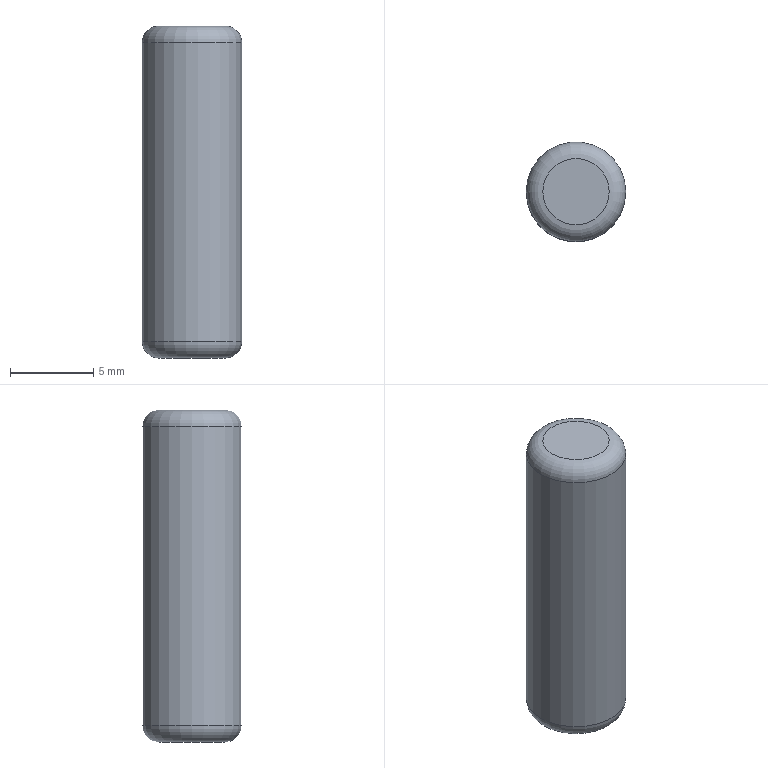Part | STEP file | 200 mesh_id710_x | 1 solid | 5 faces | box 6 x 6 x 20 mm | volume 557.999 mm3 | plane 2 | torus 2 | cylinder 1 | commonest cylinder face diameters 6 x1
STEP:
#1=CARTESIAN_POINT('',(-16807.686,-4170.269,20.));
#2=VERTEX_POINT('',#1);
#3=CARTESIAN_POINT('',(-16809.686,-4170.269,20.));
#4=DIRECTION('',(0.,0.,1.));
#5=DIRECTION('',(1.,0.,0.));
#6=AXIS2_PLACEMENT_3D('',#3,#4,#5);
#7=CIRCLE('',#6,2.);
#8=EDGE_CURVE('',#2,#2,#7,.T.);
#9=ORIENTED_EDGE('',*,*,#8,.T.);
#10=EDGE_LOOP('',(#9));
#11=FACE_OUTER_BOUND('',#10,.T.);
#12=CARTESIAN_POINT('',(-16809.686,-4170.269,20.));
#13=DIRECTION('',(0.,0.,1.));
#14=DIRECTION('',(1.,0.,0.));
#15=AXIS2_PLACEMENT_3D('',#12,#13,#14);
#16=PLANE('',#15);
#17=ADVANCED_FACE('',(#11),#16,.T.);
#18=CARTESIAN_POINT('',(-16811.686,-4170.269,0.));
#19=VERTEX_POINT('',#18);
#20=CARTESIAN_POINT('',(-16809.686,-4170.269,0.));
#21=DIRECTION('',(0.,0.,-1.));
#22=DIRECTION('',(-1.,0.,0.));
#23=AXIS2_PLACEMENT_3D('',#20,#21,#22);
#24=CIRCLE('',#23,2.);
#25=EDGE_CURVE('',#19,#19,#24,.T.);
#26=ORIENTED_EDGE('',*,*,#25,.T.);
#27=EDGE_LOOP('',(#26));
#28=FACE_OUTER_BOUND('',#27,.T.);
#29=CARTESIAN_POINT('',(-16809.686,-4170.269,0.));
#30=DIRECTION('',(0.,0.,-1.));
#31=DIRECTION('',(-1.,0.,0.));
#32=AXIS2_PLACEMENT_3D('',#29,#30,#31);
#33=PLANE('',#32);
#34=ADVANCED_FACE('',(#28),#33,.T.);
#35=CARTESIAN_POINT('',(-16812.686,-4170.269,1.));
#36=VERTEX_POINT('',#35);
#37=CARTESIAN_POINT('',(-16809.686,-4170.269,1.));
#38=DIRECTION('',(0.,0.,1.));
#39=DIRECTION('',(-1.,0.,0.));
#40=AXIS2_PLACEMENT_3D('',#37,#38,#39);
#41=CIRCLE('',#40,3.);
#42=EDGE_CURVE('',#36,#36,#41,.T.);
#43=ORIENTED_EDGE('',*,*,#42,.T.);
#44=EDGE_LOOP('',(#43));
#45=FACE_BOUND('',#44,.T.);
#46=CARTESIAN_POINT('',(-16806.686,-4170.269,19.));
#47=VERTEX_POINT('',#46);
#48=CARTESIAN_POINT('',(-16809.686,-4170.269,19.));
#49=DIRECTION('',(0.,0.,-1.));
#50=DIRECTION('',(1.,0.,0.));
#51=AXIS2_PLACEMENT_3D('',#48,#49,#50);
#52=CIRCLE('',#51,3.);
#53=EDGE_CURVE('',#47,#47,#52,.T.);
#54=ORIENTED_EDGE('',*,*,#53,.T.);
#55=EDGE_LOOP('',(#54));
#56=FACE_BOUND('',#55,.T.);
#57=CARTESIAN_POINT('',(-16809.686,-4170.269,10.));
#58=DIRECTION('',(0.,0.,1.));
#59=DIRECTION('',(1.,0.,0.));
#60=AXIS2_PLACEMENT_3D('',#57,#58,#59);
#61=CYLINDRICAL_SURFACE('',#60,3.);
#62=ADVANCED_FACE('',(#45,#56),#61,.T.);
#63=ORIENTED_EDGE('',*,*,#25,.F.);
#64=EDGE_LOOP('',(#63));
#65=FACE_BOUND('',#64,.T.);
#66=ORIENTED_EDGE('',*,*,#42,.F.);
#67=EDGE_LOOP('',(#66));
#68=FACE_BOUND('',#67,.T.);
#69=CARTESIAN_POINT('',(-16809.686,-4170.269,1.));
#70=DIRECTION('',(0.,0.,-1.));
#71=DIRECTION('',(-1.,0.,0.));
#72=AXIS2_PLACEMENT_3D('',#69,#70,#71);
#73=TOROIDAL_SURFACE('',#72,2.,1.);
#74=ADVANCED_FACE('',(#65,#68),#73,.T.);
#75=ORIENTED_EDGE('',*,*,#8,.F.);
#76=EDGE_LOOP('',(#75));
#77=FACE_BOUND('',#76,.T.);
#78=ORIENTED_EDGE('',*,*,#53,.F.);
#79=EDGE_LOOP('',(#78));
#80=FACE_BOUND('',#79,.T.);
#81=CARTESIAN_POINT('',(-16809.686,-4170.269,19.));
#82=DIRECTION('',(0.,0.,1.));
#83=DIRECTION('',(1.,0.,0.));
#84=AXIS2_PLACEMENT_3D('',#81,#82,#83);
#85=TOROIDAL_SURFACE('',#84,2.,1.);
#86=ADVANCED_FACE('',(#77,#80),#85,.T.);
#87=CLOSED_SHELL('',(#17,#34,#62,#74,#86));
#88=MANIFOLD_SOLID_BREP('',#87);
#89=(LENGTH_UNIT()NAMED_UNIT(*)SI_UNIT(.MILLI.,.METRE.));
#90=UNCERTAINTY_MEASURE_WITH_UNIT(LENGTH_MEASURE(0.00002),#89,'','');
#91=(NAMED_UNIT(*)PLANE_ANGLE_UNIT()SI_UNIT($,.RADIAN.));
#92=PLANE_ANGLE_MEASURE_WITH_UNIT(PLANE_ANGLE_MEASURE(0.01745),#91);
#93=DIMENSIONAL_EXPONENTS(0.,0.,0.,0.,0.,0.,0.);
#94=(CONVERSION_BASED_UNIT('DEGREE',#92)NAMED_UNIT(#93)PLANE_ANGLE_UNIT());
#95=(NAMED_UNIT(*)SI_UNIT($,.STERADIAN.)SOLID_ANGLE_UNIT());
#96=(GEOMETRIC_REPRESENTATION_CONTEXT(3)GLOBAL_UNCERTAINTY_ASSIGNED_CONTEXT((#90))GLOBAL_UNIT_ASSIGNED_CONTEXT((#89,#94,#95))REPRESENTATION_CONTEXT('',''));
#97=ADVANCED_BREP_SHAPE_REPRESENTATION('',(#88),#96);